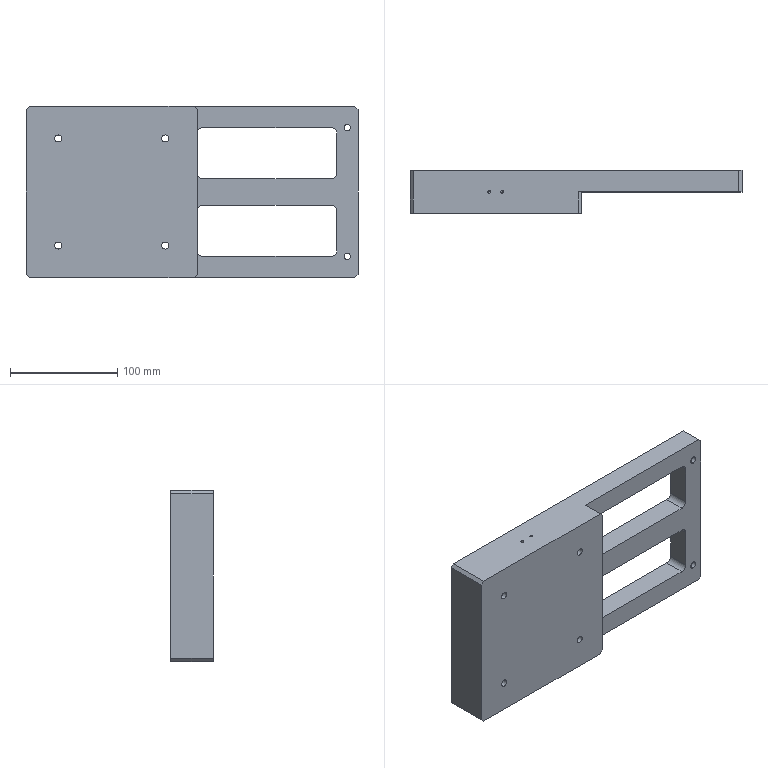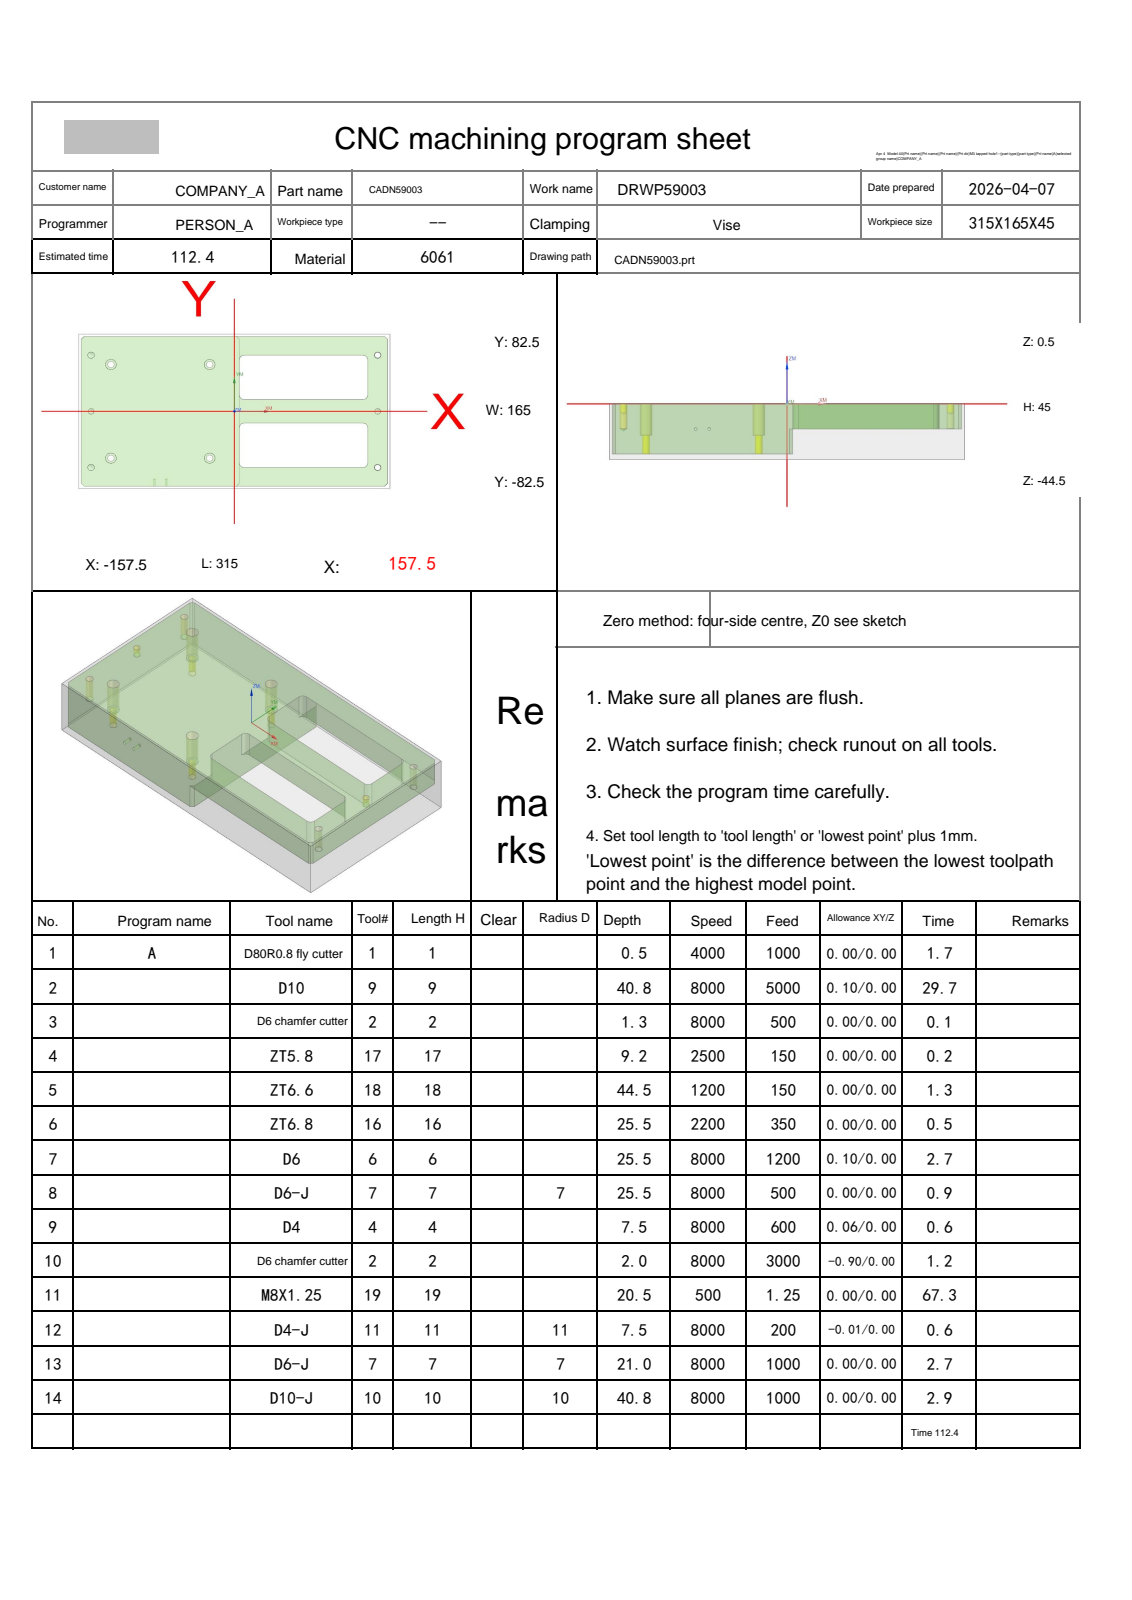NC program | NX | posted by the shop | part box 310 x 40 x 160 mm
Lines 45 to 781 of 5464:
N2 T09 M06
(D10  D=10. R=0. H=09 ce=0.10 di=0.00)
G00 G90 G54 X0.0 Y85.1 M03 S8000
G43 H09 Z20.
M08
Z.5
G01 X152. Z.376 F5000.
G02 X155.606 Y83.606 Z.373 I0.0 J-5.1
G01 X158.606 Y80.606 Z.37
G02 X160.1 Y77. Z.366 I-3.606 J-3.606
G01 Y-77. Z.241
G02 X158.606 Y-80.606 Z.238 I-5.1 J0.0
G01 X155.606 Y-83.606 Z.235
G02 X152. Y-85.1 Z.231 I-3.606 J3.606
G01 X-152. Z-.016
G02 X-155.606 Y-83.606 Z-.019 I0.0 J5.1
G01 X-158.606 Y-80.606 Z-.023
G02 X-160.1 Y-77. Z-.026 I3.606 J3.606
G01 Y77. Z-.151
G02 X-158.606 Y80.606 Z-.154 I5.1 J0.0
G01 X-155.606 Y83.606 Z-.158
G02 X-152. Y85.1 Z-.161 I3.606 J-3.606
G01 X152. Z-.408
G02 X155.606 Y83.606 Z-.411 I0.0 J-5.1
G01 X158.606 Y80.606 Z-.415
G02 X160.1 Y77. Z-.418 I-3.606 J-3.606
G01 Y-77. Z-.543
G02 X158.606 Y-80.606 Z-.547 I-5.1 J0.0
G01 X155.606 Y-83.606 Z-.55
G02 X152. Y-85.1 Z-.553 I-3.606 J3.606
G01 X-152. Z-.801
G02 X-155.606 Y-83.606 Z-.804 I0.0 J5.1
G01 X-158.606 Y-80.606 Z-.807
G02 X-160.1 Y-77. Z-.81 I3.606 J3.606
G01 Y77. Z-.936
G02 X-158.606 Y80.606 Z-.939 I5.1 J0.0
G01 X-155.606 Y83.606 Z-.942
G02 X-152. Y85.1 Z-.946 I3.606 J-3.606
G01 X152. Z-1.193
G02 X155.606 Y83.606 Z-1.196 I0.0 J-5.1
G01 X158.606 Y80.606 Z-1.2
G02 X160.1 Y77. Z-1.203 I-3.606 J-3.606
G01 Y-77. Z-1.328
G02 X158.606 Y-80.606 Z-1.331 I-5.1 J0.0
G01 X155.606 Y-83.606 Z-1.335
G02 X152. Y-85.1 Z-1.338 I-3.606 J3.606
G01 X-152. Z-1.585
G02 X-155.606 Y-83.606 Z-1.588 I0.0 J5.1
G01 X-158.606 Y-80.606 Z-1.592
G02 X-160.1 Y-77. Z-1.595 I3.606 J3.606
G01 Y77. Z-1.72
G02 X-158.606 Y80.606 Z-1.724 I5.1 J0.0
G01 X-155.606 Y83.606 Z-1.727
G02 X-152. Y85.1 Z-1.73 I3.606 J-3.606
G01 X152. Z-1.977
G02 X155.606 Y83.606 Z-1.981 I0.0 J-5.1
G01 X158.606 Y80.606 Z-1.984
G02 X160.1 Y77. Z-1.987 I-3.606 J-3.606
G01 Y-77. Z-2.113
G02 X158.606 Y-80.606 Z-2.116 I-5.1 J0.0
G01 X155.606 Y-83.606 Z-2.119
G02 X152. Y-85.1 Z-2.123 I-3.606 J3.606
G01 X-152. Z-2.37
G02 X-155.606 Y-83.606 Z-2.373 I0.0 J5.1
G01 X-158.606 Y-80.606 Z-2.376
G02 X-160.1 Y-77. Z-2.38 I3.606 J3.606
G01 Y77. Z-2.505
G02 X-158.606 Y80.606 Z-2.508 I5.1 J0.0
G01 X-155.606 Y83.606 Z-2.512
G02 X-152. Y85.1 Z-2.515 I3.606 J-3.606
G01 X152. Z-2.762
G02 X155.606 Y83.606 Z-2.765 I0.0 J-5.1
G01 X158.606 Y80.606 Z-2.769
G02 X160.1 Y77. Z-2.772 I-3.606 J-3.606
G01 Y-77. Z-2.897
G02 X158.606 Y-80.606 Z-2.9 I-5.1 J0.0
G01 X155.606 Y-83.606 Z-2.904
G02 X152. Y-85.1 Z-2.907 I-3.606 J3.606
G01 X-152. Z-3.154
G02 X-155.606 Y-83.606 Z-3.158 I0.0 J5.1
G01 X-158.606 Y-80.606 Z-3.161
G02 X-160.1 Y-77. Z-3.164 I3.606 J3.606
G01 Y77. Z-3.29
G02 X-158.606 Y80.606 Z-3.293 I5.1 J0.0
G01 X-155.606 Y83.606 Z-3.296
G02 X-152. Y85.1 Z-3.299 I3.606 J-3.606
G01 X152. Z-3.547
G02 X155.606 Y83.606 Z-3.55 I0.0 J-5.1
G01 X158.606 Y80.606 Z-3.553
G02 X160.1 Y77. Z-3.557 I-3.606 J-3.606
G01 Y-77. Z-3.682
G02 X158.606 Y-80.606 Z-3.685 I-5.1 J0.0
G01 X155.606 Y-83.606 Z-3.689
G02 X152. Y-85.1 Z-3.692 I-3.606 J3.606
G01 X-152. Z-3.939
G02 X-155.606 Y-83.606 Z-3.942 I0.0 J5.1
G01 X-158.606 Y-80.606 Z-3.946
G02 X-160.1 Y-77. Z-3.949 I3.606 J3.606
G01 Y77. Z-4.074
G02 X-158.606 Y80.606 Z-4.077 I5.1 J0.0
G01 X-155.606 Y83.606 Z-4.081
G02 X-152. Y85.1 Z-4.084 I3.606 J-3.606
G01 X152. Z-4.331
G02 X155.606 Y83.606 Z-4.335 I0.0 J-5.1
G01 X158.606 Y80.606 Z-4.338
G02 X160.1 Y77. Z-4.341 I-3.606 J-3.606
G01 Y-77. Z-4.466
G02 X158.606 Y-80.606 Z-4.47 I-5.1 J0.0
G01 X155.606 Y-83.606 Z-4.473
G02 X152. Y-85.1 Z-4.476 I-3.606 J3.606
G01 X-152. Z-4.724
G02 X-155.606 Y-83.606 Z-4.727 I0.0 J5.1
G01 X-158.606 Y-80.606 Z-4.73
G02 X-160.1 Y-77. Z-4.734 I3.606 J3.606
G01 Y77. Z-4.859
G02 X-158.606 Y80.606 Z-4.862 I5.1 J0.0
G01 X-155.606 Y83.606 Z-4.865
G02 X-152. Y85.1 Z-4.869 I3.606 J-3.606
G01 X152. Z-5.116
G02 X155.606 Y83.606 Z-5.119 I0.0 J-5.1
G01 X158.606 Y80.606 Z-5.123
G02 X160.1 Y77. Z-5.126 I-3.606 J-3.606
G01 Y-77. Z-5.251
G02 X158.606 Y-80.606 Z-5.254 I-5.1 J0.0
G01 X155.606 Y-83.606 Z-5.258
G02 X152. Y-85.1 Z-5.261 I-3.606 J3.606
G01 X-152. Z-5.508
G02 X-155.606 Y-83.606 Z-5.511 I0.0 J5.1
G01 X-158.606 Y-80.606 Z-5.515
G02 X-160.1 Y-77. Z-5.518 I3.606 J3.606
G01 Y77. Z-5.643
G02 X-158.606 Y80.606 Z-5.647 I5.1 J0.0
G01 X-155.606 Y83.606 Z-5.65
G02 X-152. Y85.1 Z-5.653 I3.606 J-3.606
G01 X152. Z-5.901
G02 X155.606 Y83.606 Z-5.904 I0.0 J-5.1
G01 X158.606 Y80.606 Z-5.907
G02 X160.1 Y77. Z-5.91 I-3.606 J-3.606
G01 Y-77. Z-6.036
G02 X158.606 Y-80.606 Z-6.039 I-5.1 J0.0
G01 X155.606 Y-83.606 Z-6.042
G02 X152. Y-85.1 Z-6.046 I-3.606 J3.606
G01 X-152. Z-6.293
G02 X-155.606 Y-83.606 Z-6.296 I0.0 J5.1
G01 X-158.606 Y-80.606 Z-6.3
G02 X-160.1 Y-77. Z-6.303 I3.606 J3.606
G01 Y77. Z-6.428
G02 X-158.606 Y80.606 Z-6.431 I5.1 J0.0
G01 X-155.606 Y83.606 Z-6.435
G02 X-152. Y85.1 Z-6.438 I3.606 J-3.606
G01 X152. Z-6.685
G02 X155.606 Y83.606 Z-6.688 I0.0 J-5.1
G01 X158.606 Y80.606 Z-6.692
G02 X160.1 Y77. Z-6.695 I-3.606 J-3.606
G01 Y-77. Z-6.82
G02 X158.606 Y-80.606 Z-6.824 I-5.1 J0.0
G01 X155.606 Y-83.606 Z-6.827
G02 X152. Y-85.1 Z-6.83 I-3.606 J3.606
G01 X-152. Z-7.077
G02 X-155.606 Y-83.606 Z-7.081 I0.0 J5.1
G01 X-158.606 Y-80.606 Z-7.084
G02 X-160.1 Y-77. Z-7.087 I3.606 J3.606
G01 Y77. Z-7.213
G02 X-158.606 Y80.606 Z-7.216 I5.1 J0.0
G01 X-155.606 Y83.606 Z-7.219
G02 X-152. Y85.1 Z-7.223 I3.606 J-3.606
G01 X152. Z-7.47
G02 X155.606 Y83.606 Z-7.473 I0.0 J-5.1
G01 X158.606 Y80.606 Z-7.476
G02 X160.1 Y77. Z-7.48 I-3.606 J-3.606
G01 Y-77. Z-7.605
G02 X158.606 Y-80.606 Z-7.608 I-5.1 J0.0
G01 X155.606 Y-83.606 Z-7.612
G02 X152. Y-85.1 Z-7.615 I-3.606 J3.606
G01 X-152. Z-7.862
G02 X-155.606 Y-83.606 Z-7.865 I0.0 J5.1
G01 X-158.606 Y-80.606 Z-7.869
G02 X-160.1 Y-77. Z-7.872 I3.606 J3.606
G01 Y77. Z-7.997
G02 X-158.606 Y80.606 Z-8. I5.1 J0.0
G01 X-155.606 Y83.606 Z-8.004
G02 X-152. Y85.1 Z-8.007 I3.606 J-3.606
G01 X152. Z-8.254
G02 X155.606 Y83.606 Z-8.258 I0.0 J-5.1
G01 X158.606 Y80.606 Z-8.261
G02 X160.1 Y77. Z-8.264 I-3.606 J-3.606
G01 Y-77. Z-8.39
G02 X158.606 Y-80.606 Z-8.393 I-5.1 J0.0
G01 X155.606 Y-83.606 Z-8.396
G02 X152. Y-85.1 Z-8.399 I-3.606 J3.606
G01 X-152. Z-8.647
G02 X-155.606 Y-83.606 Z-8.65 I0.0 J5.1
G01 X-158.606 Y-80.606 Z-8.653
G02 X-160.1 Y-77. Z-8.657 I3.606 J3.606
G01 Y77. Z-8.782
G02 X-158.606 Y80.606 Z-8.785 I5.1 J0.0
G01 X-155.606 Y83.606 Z-8.789
G02 X-152. Y85.1 Z-8.792 I3.606 J-3.606
G01 X152. Z-9.039
G02 X155.606 Y83.606 Z-9.042 I0.0 J-5.1
G01 X158.606 Y80.606 Z-9.046
G02 X160.1 Y77. Z-9.049 I-3.606 J-3.606
G01 Y-77. Z-9.174
G02 X158.606 Y-80.606 Z-9.177 I-5.1 J0.0
G01 X155.606 Y-83.606 Z-9.181
G02 X152. Y-85.1 Z-9.184 I-3.606 J3.606
G01 X-152. Z-9.431
G02 X-155.606 Y-83.606 Z-9.435 I0.0 J5.1
G01 X-158.606 Y-80.606 Z-9.438
G02 X-160.1 Y-77. Z-9.441 I3.606 J3.606
G01 Y77. Z-9.566
G02 X-158.606 Y80.606 Z-9.57 I5.1 J0.0
G01 X-155.606 Y83.606 Z-9.573
G02 X-152. Y85.1 Z-9.576 I3.606 J-3.606
G01 X152. Z-9.824
G02 X155.606 Y83.606 Z-9.827 I0.0 J-5.1
G01 X158.606 Y80.606 Z-9.83
G02 X160.1 Y77. Z-9.834 I-3.606 J-3.606
G01 Y-77. Z-9.959
G02 X158.606 Y-80.606 Z-9.962 I-5.1 J0.0
G01 X155.606 Y-83.606 Z-9.965
G02 X152. Y-85.1 Z-9.969 I-3.606 J3.606
G01 X-152. Z-10.216
G02 X-155.606 Y-83.606 Z-10.219 I0.0 J5.1
G01 X-158.606 Y-80.606 Z-10.223
G02 X-160.1 Y-77. Z-10.226 I3.606 J3.606
G01 Y77. Z-10.351
G02 X-158.606 Y80.606 Z-10.354 I5.1 J0.0
G01 X-155.606 Y83.606 Z-10.358
G02 X-152. Y85.1 Z-10.361 I3.606 J-3.606
G01 X152. Z-10.608
G02 X155.606 Y83.606 Z-10.611 I0.0 J-5.1
G01 X158.606 Y80.606 Z-10.615
G02 X160.1 Y77. Z-10.618 I-3.606 J-3.606
G01 Y-77. Z-10.743
G02 X158.606 Y-80.606 Z-10.747 I-5.1 J0.0
G01 X155.606 Y-83.606 Z-10.75
G02 X152. Y-85.1 Z-10.753 I-3.606 J3.606
G01 X-152. Z-11.001
G02 X-155.606 Y-83.606 Z-11.004 I0.0 J5.1
G01 X-158.606 Y-80.606 Z-11.007
G02 X-160.1 Y-77. Z-11.01 I3.606 J3.606
G01 Y77. Z-11.136
G02 X-158.606 Y80.606 Z-11.139 I5.1 J0.0
G01 X-155.606 Y83.606 Z-11.142
G02 X-152. Y85.1 Z-11.146 I3.606 J-3.606
G01 X152. Z-11.393
G02 X155.606 Y83.606 Z-11.396 I0.0 J-5.1
G01 X158.606 Y80.606 Z-11.4
G02 X160.1 Y77. Z-11.403 I-3.606 J-3.606
G01 Y-77. Z-11.528
G02 X158.606 Y-80.606 Z-11.531 I-5.1 J0.0
G01 X155.606 Y-83.606 Z-11.535
G02 X152. Y-85.1 Z-11.538 I-3.606 J3.606
G01 X-152. Z-11.785
G02 X-155.606 Y-83.606 Z-11.788 I0.0 J5.1
G01 X-158.606 Y-80.606 Z-11.792
G02 X-160.1 Y-77. Z-11.795 I3.606 J3.606
G01 Y77. Z-11.92
G02 X-158.606 Y80.606 Z-11.924 I5.1 J0.0
G01 X-155.606 Y83.606 Z-11.927
G02 X-152. Y85.1 Z-11.93 I3.606 J-3.606
G01 X152. Z-12.177
G02 X155.606 Y83.606 Z-12.181 I0.0 J-5.1
G01 X158.606 Y80.606 Z-12.184
G02 X160.1 Y77. Z-12.187 I-3.606 J-3.606
G01 Y-77. Z-12.313
G02 X158.606 Y-80.606 Z-12.316 I-5.1 J0.0
G01 X155.606 Y-83.606 Z-12.319
G02 X152. Y-85.1 Z-12.323 I-3.606 J3.606
G01 X-152. Z-12.57
G02 X-155.606 Y-83.606 Z-12.573 I0.0 J5.1
G01 X-158.606 Y-80.606 Z-12.576
G02 X-160.1 Y-77. Z-12.58 I3.606 J3.606
G01 Y77. Z-12.705
G02 X-158.606 Y80.606 Z-12.708 I5.1 J0.0
G01 X-155.606 Y83.606 Z-12.712
G02 X-152. Y85.1 Z-12.715 I3.606 J-3.606
G01 X152. Z-12.962
G02 X155.606 Y83.606 Z-12.965 I0.0 J-5.1
G01 X158.606 Y80.606 Z-12.969
G02 X160.1 Y77. Z-12.972 I-3.606 J-3.606
G01 Y-77. Z-13.097
G02 X158.606 Y-80.606 Z-13.1 I-5.1 J0.0
G01 X155.606 Y-83.606 Z-13.104
G02 X152. Y-85.1 Z-13.107 I-3.606 J3.606
G01 X-152. Z-13.354
G02 X-155.606 Y-83.606 Z-13.358 I0.0 J5.1
G01 X-158.606 Y-80.606 Z-13.361
G02 X-160.1 Y-77. Z-13.364 I3.606 J3.606
G01 Y77. Z-13.49
G02 X-158.606 Y80.606 Z-13.493 I5.1 J0.0
G01 X-155.606 Y83.606 Z-13.496
G02 X-152. Y85.1 Z-13.499 I3.606 J-3.606
G01 X152. Z-13.747
G02 X155.606 Y83.606 Z-13.75 I0.0 J-5.1
G01 X158.606 Y80.606 Z-13.753
G02 X160.1 Y77. Z-13.757 I-3.606 J-3.606
G01 Y-77. Z-13.882
G02 X158.606 Y-80.606 Z-13.885 I-5.1 J0.0
G01 X155.606 Y-83.606 Z-13.889
G02 X152. Y-85.1 Z-13.892 I-3.606 J3.606
G01 X-152. Z-14.139
G02 X-155.606 Y-83.606 Z-14.142 I0.0 J5.1
G01 X-158.606 Y-80.606 Z-14.146
G02 X-160.1 Y-77. Z-14.149 I3.606 J3.606
G01 Y77. Z-14.274
G02 X-158.606 Y80.606 Z-14.277 I5.1 J0.0
G01 X-155.606 Y83.606 Z-14.281
G02 X-152. Y85.1 Z-14.284 I3.606 J-3.606
G01 X152. Z-14.531
G02 X155.606 Y83.606 Z-14.535 I0.0 J-5.1
G01 X158.606 Y80.606 Z-14.538
G02 X160.1 Y77. Z-14.541 I-3.606 J-3.606
G01 Y-77. Z-14.666
G02 X158.606 Y-80.606 Z-14.67 I-5.1 J0.0
G01 X155.606 Y-83.606 Z-14.673
G02 X152. Y-85.1 Z-14.676 I-3.606 J3.606
G01 X-152. Z-14.924
G02 X-155.606 Y-83.606 Z-14.927 I0.0 J5.1
G01 X-158.606 Y-80.606 Z-14.93
G02 X-160.1 Y-77. Z-14.934 I3.606 J3.606
G01 Y77. Z-15.059
G02 X-158.606 Y80.606 Z-15.062 I5.1 J0.0
G01 X-155.606 Y83.606 Z-15.065
G02 X-152. Y85.1 Z-15.069 I3.606 J-3.606
G01 X152. Z-15.316
G02 X155.606 Y83.606 Z-15.319 I0.0 J-5.1
G01 X158.606 Y80.606 Z-15.323
G02 X160.1 Y77. Z-15.326 I-3.606 J-3.606
G01 Y-77. Z-15.451
G02 X158.606 Y-80.606 Z-15.454 I-5.1 J0.0
G01 X155.606 Y-83.606 Z-15.458
G02 X152. Y-85.1 Z-15.461 I-3.606 J3.606
G01 X-152. Z-15.708
G02 X-155.606 Y-83.606 Z-15.711 I0.0 J5.1
G01 X-158.606 Y-80.606 Z-15.715
G02 X-160.1 Y-77. Z-15.718 I3.606 J3.606
G01 Y77. Z-15.843
G02 X-158.606 Y80.606 Z-15.847 I5.1 J0.0
G01 X-155.606 Y83.606 Z-15.85
G02 X-152. Y85.1 Z-15.853 I3.606 J-3.606
G01 X152. Z-16.101
G02 X155.606 Y83.606 Z-16.104 I0.0 J-5.1
G01 X158.606 Y80.606 Z-16.107
G02 X160.1 Y77. Z-16.11 I-3.606 J-3.606
G01 Y-77. Z-16.236
G02 X158.606 Y-80.606 Z-16.239 I-5.1 J0.0
G01 X155.606 Y-83.606 Z-16.242
G02 X152. Y-85.1 Z-16.246 I-3.606 J3.606
G01 X-152. Z-16.493
G02 X-155.606 Y-83.606 Z-16.496 I0.0 J5.1
G01 X-158.606 Y-80.606 Z-16.5
G02 X-160.1 Y-77. Z-16.503 I3.606 J3.606
G01 Y77. Z-16.628
G02 X-158.606 Y80.606 Z-16.631 I5.1 J0.0
G01 X-155.606 Y83.606 Z-16.635
G02 X-152. Y85.1 Z-16.638 I3.606 J-3.606
G01 X152. Z-16.885
G02 X155.606 Y83.606 Z-16.888 I0.0 J-5.1
G01 X158.606 Y80.606 Z-16.892
G02 X160.1 Y77. Z-16.895 I-3.606 J-3.606
G01 Y-77. Z-17.02
G02 X158.606 Y-80.606 Z-17.024 I-5.1 J0.0
G01 X155.606 Y-83.606 Z-17.027
G02 X152. Y-85.1 Z-17.03 I-3.606 J3.606
G01 X-152. Z-17.277
G02 X-155.606 Y-83.606 Z-17.281 I0.0 J5.1
G01 X-158.606 Y-80.606 Z-17.284
G02 X-160.1 Y-77. Z-17.287 I3.606 J3.606
G01 Y77. Z-17.413
G02 X-158.606 Y80.606 Z-17.416 I5.1 J0.0
G01 X-155.606 Y83.606 Z-17.419
G02 X-152. Y85.1 Z-17.423 I3.606 J-3.606
G01 X152. Z-17.67
G02 X155.606 Y83.606 Z-17.673 I0.0 J-5.1
G01 X158.606 Y80.606 Z-17.676
G02 X160.1 Y77. Z-17.68 I-3.606 J-3.606
G01 Y-77. Z-17.805
G02 X158.606 Y-80.606 Z-17.808 I-5.1 J0.0
G01 X155.606 Y-83.606 Z-17.812
G02 X152. Y-85.1 Z-17.815 I-3.606 J3.606
G01 X-152. Z-18.062
G02 X-155.606 Y-83.606 Z-18.065 I0.0 J5.1
G01 X-158.606 Y-80.606 Z-18.069
G02 X-160.1 Y-77. Z-18.072 I3.606 J3.606
G01 Y77. Z-18.197
G02 X-158.606 Y80.606 Z-18.2 I5.1 J0.0
G01 X-155.606 Y83.606 Z-18.204
G02 X-152. Y85.1 Z-18.207 I3.606 J-3.606
G01 X152. Z-18.454
G02 X155.606 Y83.606 Z-18.458 I0.0 J-5.1
G01 X158.606 Y80.606 Z-18.461
G02 X160.1 Y77. Z-18.464 I-3.606 J-3.606
G01 Y-77. Z-18.59
G02 X158.606 Y-80.606 Z-18.593 I-5.1 J0.0
G01 X155.606 Y-83.606 Z-18.596
G02 X152. Y-85.1 Z-18.599 I-3.606 J3.606
G01 X-152. Z-18.847
G02 X-155.606 Y-83.606 Z-18.85 I0.0 J5.1
G01 X-158.606 Y-80.606 Z-18.853
G02 X-160.1 Y-77. Z-18.857 I3.606 J3.606
G01 Y77. Z-18.982
G02 X-158.606 Y80.606 Z-18.985 I5.1 J0.0
G01 X-155.606 Y83.606 Z-18.989
G02 X-152. Y85.1 Z-18.992 I3.606 J-3.606
G01 X152. Z-19.239
G02 X155.606 Y83.606 Z-19.242 I0.0 J-5.1
G01 X158.606 Y80.606 Z-19.246
G02 X160.1 Y77. Z-19.249 I-3.606 J-3.606
G01 Y-77. Z-19.374
G02 X158.606 Y-80.606 Z-19.377 I-5.1 J0.0
G01 X155.606 Y-83.606 Z-19.381
G02 X152. Y-85.1 Z-19.384 I-3.606 J3.606
G01 X-152. Z-19.631
G02 X-155.606 Y-83.606 Z-19.635 I0.0 J5.1
G01 X-158.606 Y-80.606 Z-19.638
G02 X-160.1 Y-77. Z-19.641 I3.606 J3.606
G01 Y77. Z-19.766
G02 X-158.606 Y80.606 Z-19.77 I5.1 J0.0
G01 X-155.606 Y83.606 Z-19.773
G02 X-152. Y85.1 Z-19.776 I3.606 J-3.606
G01 X152. Z-20.024
G02 X155.606 Y83.606 Z-20.027 I0.0 J-5.1
G01 X158.606 Y80.606 Z-20.03
G02 X160.1 Y77. Z-20.034 I-3.606 J-3.606
G01 Y-77. Z-20.159
G02 X158.606 Y-80.606 Z-20.162 I-5.1 J0.0
G01 X155.606 Y-83.606 Z-20.165
G02 X152. Y-85.1 Z-20.169 I-3.606 J3.606
G01 X-152. Z-20.416
G02 X-155.606 Y-83.606 Z-20.419 I0.0 J5.1
G01 X-158.606 Y-80.606 Z-20.423
G02 X-160.1 Y-77. Z-20.426 I3.606 J3.606
G01 Y77. Z-20.551
G02 X-158.606 Y80.606 Z-20.554 I5.1 J0.0
G01 X-155.606 Y83.606 Z-20.558
G02 X-152. Y85.1 Z-20.561 I3.606 J-3.606
G01 X152. Z-20.808
G02 X155.606 Y83.606 Z-20.811 I0.0 J-5.1
G01 X158.606 Y80.606 Z-20.815
G02 X160.1 Y77. Z-20.818 I-3.606 J-3.606
G01 Y-77. Z-20.943
G02 X158.606 Y-80.606 Z-20.947 I-5.1 J0.0
G01 X155.606 Y-83.606 Z-20.95
G02 X152. Y-85.1 Z-20.953 I-3.606 J3.606
G01 X-152. Z-21.201
G02 X-155.606 Y-83.606 Z-21.204 I0.0 J5.1
G01 X-158.606 Y-80.606 Z-21.207
G02 X-160.1 Y-77. Z-21.21 I3.606 J3.606
G01 Y77. Z-21.336
G02 X-158.606 Y80.606 Z-21.339 I5.1 J0.0
G01 X-155.606 Y83.606 Z-21.342
G02 X-152. Y85.1 Z-21.346 I3.606 J-3.606
G01 X152. Z-21.593
G02 X155.606 Y83.606 Z-21.596 I0.0 J-5.1
G01 X158.606 Y80.606 Z-21.6
G02 X160.1 Y77. Z-21.603 I-3.606 J-3.606
G01 Y-77. Z-21.728
G02 X158.606 Y-80.606 Z-21.731 I-5.1 J0.0
G01 X155.606 Y-83.606 Z-21.735
G02 X152. Y-85.1 Z-21.738 I-3.606 J3.606
G01 X-152. Z-21.985
G02 X-155.606 Y-83.606 Z-21.988 I0.0 J5.1
G01 X-158.606 Y-80.606 Z-21.992
G02 X-160.1 Y-77. Z-21.995 I3.606 J3.606
G01 Y77. Z-22.12
G02 X-158.606 Y80.606 Z-22.124 I5.1 J0.0
G01 X-155.606 Y83.606 Z-22.127
G02 X-152. Y85.1 Z-22.13 I3.606 J-3.606
G01 X152. Z-22.377
G02 X155.606 Y83.606 Z-22.381 I0.0 J-5.1
G01 X158.606 Y80.606 Z-22.384
G02 X160.1 Y77. Z-22.387 I-3.606 J-3.606
G01 Y-77. Z-22.513
G02 X158.606 Y-80.606 Z-22.516 I-5.1 J0.0
G01 X155.606 Y-83.606 Z-22.519
G02 X152. Y-85.1 Z-22.523 I-3.606 J3.606
G01 X-152. Z-22.77
G02 X-155.606 Y-83.606 Z-22.773 I0.0 J5.1
G01 X-158.606 Y-80.606 Z-22.776
G02 X-160.1 Y-77. Z-22.78 I3.606 J3.606
G01 Y77. Z-22.905
G02 X-158.606 Y80.606 Z-22.908 I5.1 J0.0
G01 X-155.606 Y83.606 Z-22.912
G02 X-152. Y85.1 Z-22.915 I3.606 J-3.606
G01 X152. Z-23.162
G02 X155.606 Y83.606 Z-23.165 I0.0 J-5.1
G01 X158.606 Y80.606 Z-23.169
G02 X160.1 Y77. Z-23.172 I-3.606 J-3.606
G01 Y-77. Z-23.297
G02 X158.606 Y-80.606 Z-23.3 I-5.1 J0.0
G01 X155.606 Y-83.606 Z-23.304
G02 X152. Y-85.1 Z-23.307 I-3.606 J3.606
G01 X-152. Z-23.554
G02 X-155.606 Y-83.606 Z-23.558 I0.0 J5.1
G01 X-158.606 Y-80.606 Z-23.561
G02 X-160.1 Y-77. Z-23.564 I3.606 J3.606
G01 Y77. Z-23.69
G02 X-158.606 Y80.606 Z-23.693 I5.1 J0.0
G01 X-155.606 Y83.606 Z-23.696
G02 X-152. Y85.1 Z-23.699 I3.606 J-3.606
G01 X152. Z-23.947
G02 X155.606 Y83.606 Z-23.95 I0.0 J-5.1
G01 X158.606 Y80.606 Z-23.953
G02 X160.1 Y77. Z-23.957 I-3.606 J-3.606
G01 Y-77. Z-24.082
G02 X158.606 Y-80.606 Z-24.085 I-5.1 J0.0
G01 X155.606 Y-83.606 Z-24.089
G02 X152. Y-85.1 Z-24.092 I-3.606 J3.606
G01 X-152. Z-24.339
G02 X-155.606 Y-83.606 Z-24.342 I0.0 J5.1
G01 X-158.606 Y-80.606 Z-24.346
G02 X-160.1 Y-77. Z-24.349 I3.606 J3.606
G01 Y77. Z-24.474
G02 X-158.606 Y80.606 Z-24.477 I5.1 J0.0
G01 X-155.606 Y83.606 Z-24.481
G02 X-152. Y85.1 Z-24.484 I3.606 J-3.606
G01 X152. Z-24.731
G02 X155.606 Y83.606 Z-24.735 I0.0 J-5.1
G01 X158.606 Y80.606 Z-24.738
G02 X160.1 Y77. Z-24.741 I-3.606 J-3.606
G01 Y-77. Z-24.866
G02 X158.606 Y-80.606 Z-24.87 I-5.1 J0.0
G01 X155.606 Y-83.606 Z-24.873
G02 X152. Y-85.1 Z-24.876 I-3.606 J3.606
G01 X-152. Z-25.124
G02 X-155.606 Y-83.606 Z-25.127 I0.0 J5.1
G01 X-158.606 Y-80.606 Z-25.13
G02 X-160.1 Y-77. Z-25.134 I3.606 J3.606
G01 Y77. Z-25.259
G02 X-158.606 Y80.606 Z-25.262 I5.1 J0.0
G01 X-155.606 Y83.606 Z-25.265
G02 X-152. Y85.1 Z-25.269 I3.606 J-3.606
G01 X152. Z-25.516
G02 X155.606 Y83.606 Z-25.519 I0.0 J-5.1
G01 X158.606 Y80.606 Z-25.523
G02 X160.1 Y77. Z-25.526 I-3.606 J-3.606
G01 Y-77. Z-25.651
G02 X158.606 Y-80.606 Z-25.654 I-5.1 J0.0
G01 X155.606 Y-83.606 Z-25.658
G02 X152. Y-85.1 Z-25.661 I-3.606 J3.606
G01 X-152. Z-25.908
G02 X-155.606 Y-83.606 Z-25.911 I0.0 J5.1
G01 X-158.606 Y-80.606 Z-25.915
G02 X-160.1 Y-77. Z-25.918 I3.606 J3.606
G01 Y77. Z-26.043
G02 X-158.606 Y80.606 Z-26.047 I5.1 J0.0
G01 X-155.606 Y83.606 Z-26.05
G02 X-152. Y85.1 Z-26.053 I3.606 J-3.606
G01 X152. Z-26.301
G02 X155.606 Y83.606 Z-26.304 I0.0 J-5.1
G01 X158.606 Y80.606 Z-26.307
G02 X160.1 Y77. Z-26.31 I-3.606 J-3.606
G01 Y-77. Z-26.436
G02 X158.606 Y-80.606 Z-26.439 I-5.1 J0.0
G01 X155.606 Y-83.606 Z-26.442
G02 X152. Y-85.1 Z-26.446 I-3.606 J3.606
G01 X-152. Z-26.693
G02 X-155.606 Y-83.606 Z-26.696 I0.0 J5.1
G01 X-158.606 Y-80.606 Z-26.7
G02 X-160.1 Y-77. Z-26.703 I3.606 J3.606
G01 Y77. Z-26.828
G02 X-158.606 Y80.606 Z-26.831 I5.1 J0.0
G01 X-155.606 Y83.606 Z-26.835
G02 X-152. Y85.1 Z-26.838 I3.606 J-3.606
G01 X152. Z-27.085
G02 X155.606 Y83.606 Z-27.088 I0.0 J-5.1
G01 X158.606 Y80.606 Z-27.092
G02 X160.1 Y77. Z-27.095 I-3.606 J-3.606
G01 Y-77. Z-27.22
G02 X158.606 Y-80.606 Z-27.224 I-5.1 J0.0
G01 X155.606 Y-83.606 Z-27.227
G02 X152. Y-85.1 Z-27.23 I-3.606 J3.606
G01 X-152. Z-27.477
G02 X-155.606 Y-83.606 Z-27.481 I0.0 J5.1
G01 X-158.606 Y-80.606 Z-27.484
G02 X-160.1 Y-77. Z-27.487 I3.606 J3.606
G01 Y77. Z-27.613
G02 X-158.606 Y80.606 Z-27.616 I5.1 J0.0
G01 X-155.606 Y83.606 Z-27.619
G02 X-152. Y85.1 Z-27.623 I3.606 J-3.606
G01 X152. Z-27.87
G02 X155.606 Y83.606 Z-27.873 I0.0 J-5.1
G01 X158.606 Y80.606 Z-27.876
G02 X160.1 Y77. Z-27.88 I-3.606 J-3.606
G01 Y-77. Z-28.005
G02 X158.606 Y-80.606 Z-28.008 I-5.1 J0.0
G01 X155.606 Y-83.606 Z-28.012
G02 X152. Y-85.1 Z-28.015 I-3.606 J3.606
G01 X-152. Z-28.262
G02 X-155.606 Y-83.606 Z-28.265 I0.0 J5.1
G01 X-158.606 Y-80.606 Z-28.269
G02 X-160.1 Y-77. Z-28.272 I3.606 J3.606
G01 Y77. Z-28.397
G02 X-158.606 Y80.606 Z-28.4 I5.1 J0.0
G01 X-155.606 Y83.606 Z-28.404
G02 X-152. Y85.1 Z-28.407 I3.606 J-3.606
G01 X152. Z-28.654
G02 X155.606 Y83.606 Z-28.658 I0.0 J-5.1
G01 X158.606 Y80.606 Z-28.661
G02 X160.1 Y77. Z-28.664 I-3.606 J-3.606
G01 Y-77. Z-28.79
G02 X158.606 Y-80.606 Z-28.793 I-5.1 J0.0
G01 X155.606 Y-83.606 Z-28.796
G02 X152. Y-85.1 Z-28.799 I-3.606 J3.606
G01 X-152. Z-29.047
G02 X-155.606 Y-83.606 Z-29.05 I0.0 J5.1
G01 X-158.606 Y-80.606 Z-29.053
G02 X-160.1 Y-77. Z-29.057 I3.606 J3.606
G01 Y77. Z-29.182
G02 X-158.606 Y80.606 Z-29.185 I5.1 J0.0
G01 X-155.606 Y83.606 Z-29.189
G02 X-152. Y85.1 Z-29.192 I3.606 J-3.606
G01 X152. Z-29.439
G02 X155.606 Y83.606 Z-29.442 I0.0 J-5.1
G01 X158.606 Y80.606 Z-29.446
G02 X160.1 Y77. Z-29.449 I-3.606 J-3.606
G01 Y-77. Z-29.574
G02 X158.606 Y-80.606 Z-29.577 I-5.1 J0.0
G01 X155.606 Y-83.606 Z-29.581
G02 X152. Y-85.1 Z-29.584 I-3.606 J3.606
G01 X-152. Z-29.831
G02 X-155.606 Y-83.606 Z-29.835 I0.0 J5.1
G01 X-158.606 Y-80.606 Z-29.838
G02 X-160.1 Y-77. Z-29.841 I3.606 J3.606
G01 Y77. Z-29.966
G02 X-158.606 Y80.606 Z-29.97 I5.1 J0.0
G01 X-155.606 Y83.606 Z-29.973
G02 X-152. Y85.1 Z-29.976 I3.606 J-3.606
G01 X152. Z-30.224
G02 X155.606 Y83.606 Z-30.227 I0.0 J-5.1
G01 X158.606 Y80.606 Z-30.23
G02 X160.1 Y77. Z-30.234 I-3.606 J-3.606
G01 Y-77. Z-30.359
G02 X158.606 Y-80.606 Z-30.362 I-5.1 J0.0
G01 X155.606 Y-83.606 Z-30.365
G02 X152. Y-85.1 Z-30.369 I-3.606 J3.606
G01 X-152. Z-30.616
G02 X-155.606 Y-83.606 Z-30.619 I0.0 J5.1
G01 X-158.606 Y-80.606 Z-30.623
G02 X-160.1 Y-77. Z-30.626 I3.606 J3.606
G01 Y77. Z-30.751
G02 X-158.606 Y80.606 Z-30.754 I5.1 J0.0
G01 X-155.606 Y83.606 Z-30.758
G02 X-152. Y85.1 Z-30.761 I3.606 J-3.606
G01 X152. Z-31.008
G02 X155.606 Y83.606 Z-31.011 I0.0 J-5.1
G01 X158.606 Y80.606 Z-31.015
G02 X160.1 Y77. Z-31.018 I-3.606 J-3.606
G01 Y-77. Z-31.143
G02 X158.606 Y-80.606 Z-31.147 I-5.1 J0.0
G01 X155.606 Y-83.606 Z-31.15
G02 X152. Y-85.1 Z-31.153 I-3.606 J3.606
G01 X-152. Z-31.401
G02 X-155.606 Y-83.606 Z-31.404 I0.0 J5.1
G01 X-158.606 Y-80.606 Z-31.407
G02 X-160.1 Y-77. Z-31.41 I3.606 J3.606
G01 Y77. Z-31.536
G02 X-158.606 Y80.606 Z-31.539 I5.1 J0.0
G01 X-155.606 Y83.606 Z-31.542
G02 X-152. Y85.1 Z-31.546 I3.606 J-3.606
G01 X152. Z-31.793
G02 X155.606 Y83.606 Z-31.796 I0.0 J-5.1
G01 X158.606 Y80.606 Z-31.8
G02 X160.1 Y77. Z-31.803 I-3.606 J-3.606
G01 Y-77. Z-31.928
G02 X158.606 Y-80.606 Z-31.931 I-5.1 J0.0
G01 X155.606 Y-83.606 Z-31.935
G02 X152. Y-85.1 Z-31.938 I-3.606 J3.606
G01 X-152. Z-32.185
G02 X-155.606 Y-83.606 Z-32.188 I0.0 J5.1
G01 X-158.606 Y-80.606 Z-32.192
G02 X-160.1 Y-77. Z-32.195 I3.606 J3.606
G01 Y77. Z-32.32
G02 X-158.606 Y80.606 Z-32.324 I5.1 J0.0
G01 X-155.606 Y83.606 Z-32.327
G02 X-152. Y85.1 Z-32.33 I3.606 J-3.606
G01 X152. Z-32.577
G02 X155.606 Y83.606 Z-32.581 I0.0 J-5.1
G01 X158.606 Y80.606 Z-32.584
G02 X160.1 Y77. Z-32.587 I-3.606 J-3.606
G01 Y-77. Z-32.713
G02 X158.606 Y-80.606 Z-32.716 I-5.1 J0.0
G01 X155.606 Y-83.606 Z-32.719
G02 X152. Y-85.1 Z-32.723 I-3.606 J3.606
G01 X-152. Z-32.97
G02 X-155.606 Y-83.606 Z-32.973 I0.0 J5.1
G01 X-158.606 Y-80.606 Z-32.976
G02 X-160.1 Y-77. Z-32.98 I3.606 J3.606
G01 Y77. Z-33.105
G02 X-158.606 Y80.606 Z-33.108 I5.1 J0.0
G01 X-155.606 Y83.606 Z-33.112
G02 X-152. Y85.1 Z-33.115 I3.606 J-3.606
G01 X152. Z-33.362
G02 X155.606 Y83.606 Z-33.365 I0.0 J-5.1
G01 X158.606 Y80.606 Z-33.369
G02 X160.1 Y77. Z-33.372 I-3.606 J-3.606
G01 Y-77. Z-33.497
G02 X158.606 Y-80.606 Z-33.5 I-5.1 J0.0
G01 X155.606 Y-83.606 Z-33.504
G02 X152. Y-85.1 Z-33.507 I-3.606 J3.606
G01 X-152. Z-33.754
G02 X-155.606 Y-83.606 Z-33.758 I0.0 J5.1
G01 X-158.606 Y-80.606 Z-33.761
G02 X-160.1 Y-77. Z-33.764 I3.606 J3.606
G01 Y77. Z-33.89
G02 X-158.606 Y80.606 Z-33.893 I5.1 J0.0
G01 X-155.606 Y83.606 Z-33.896
G02 X-152. Y85.1 Z-33.899 I3.606 J-3.606
G01 X152. Z-34.147
G02 X155.606 Y83.606 Z-34.15 I0.0 J-5.1
G01 X158.606 Y80.606 Z-34.153
G02 X160.1 Y77. Z-34.157 I-3.606 J-3.606
G01 Y-77. Z-34.282
G02 X158.606 Y-80.606 Z-34.285 I-5.1 J0.0
G01 X155.606 Y-83.606 Z-34.289
G02 X152. Y-85.1 Z-34.292 I-3.606 J3.606
G01 X-152. Z-34.539
G02 X-155.606 Y-83.606 Z-34.542 I0.0 J5.1
G01 X-158.606 Y-80.606 Z-34.546
G02 X-160.1 Y-77. Z-34.549 I3.606 J3.606
G01 Y77. Z-34.674
G02 X-158.606 Y80.606 Z-34.677 I5.1 J0.0
G01 X-155.606 Y83.606 Z-34.681
G02 X-152. Y85.1 Z-34.684 I3.606 J-3.606
G01 X152. Z-34.931
G02 X155.606 Y83.606 Z-34.935 I0.0 J-5.1
G01 X158.606 Y80.606 Z-34.938
G02 X160.1 Y77. Z-34.941 I-3.606 J-3.606
G01 Y-77. Z-35.066
G02 X158.606 Y-80.606 Z-35.07 I-5.1 J0.0
G01 X155.606 Y-83.606 Z-35.073
G02 X152. Y-85.1 Z-35.076 I-3.606 J3.606
G01 X-152. Z-35.324
G02 X-155.606 Y-83.606 Z-35.327 I0.0 J5.1
G01 X-158.606 Y-80.606 Z-35.33